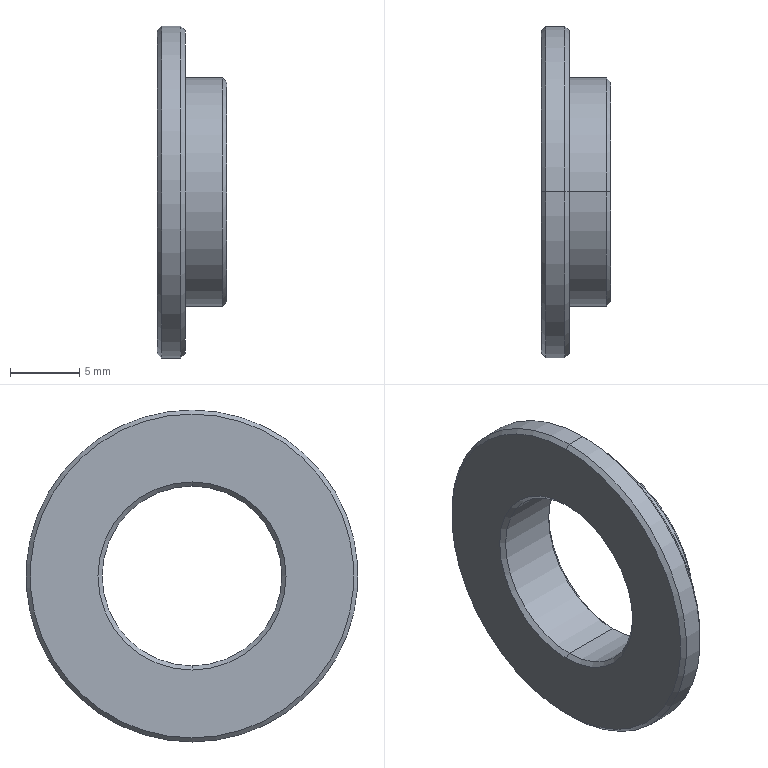Part | STEP file | ftcm_d16_5_h24_v13_0_t2_0_l5_0_2_03 | 1 solid | 19 faces | box 5 x 24 x 24 mm | volume 869.825 mm3 | cone 10 | cylinder 6 | plane 3 | commonest cylinder face diameters 13 x2 16.5 x2 24 x2
STEP:
#1=CARTESIAN_POINT('',(0.,0.,0.));
#2=DIRECTION('',(0.,0.,1.));
#3=DIRECTION('',(1.,0.,0.));
#4=AXIS2_PLACEMENT_3D('',#1,#2,#3);
#5=CARTESIAN_POINT('',(0.,0.,11.7));
#6=VERTEX_POINT('',#5);
#7=CARTESIAN_POINT('',(0.,0.,-11.7));
#8=VERTEX_POINT('',#7);
#9=CARTESIAN_POINT('',(0.,0.,0.));
#10=DIRECTION('',(-1.,0.,0.));
#11=DIRECTION('',(0.,0.,-1.));
#12=AXIS2_PLACEMENT_3D('',#9,#10,#11);
#13=CIRCLE('',#12,11.7);
#14=CARTESIAN_POINT('',(0.3,0.,0.));
#15=DIRECTION('',(1.,0.,0.));
#16=DIRECTION('',(0.,0.,-1.));
#17=AXIS2_PLACEMENT_3D('',#14,#15,#16);
#18=CONICAL_SURFACE('',#17,12.,0.7854);
#19=CARTESIAN_POINT('',(6.283,-0.3));
#20=DIRECTION('',(-1.,0.));
#21=VECTOR('',#20,1.);
#22=LINE('',#19,#21);
#23=(GEOMETRIC_REPRESENTATION_CONTEXT(2)PARAMETRIC_REPRESENTATION_CONTEXT()REPRESENTATION_CONTEXT('',''));
#24=DEFINITIONAL_REPRESENTATION('',(#22),#23);
#25=PCURVE('',#18,#24);
#26=CARTESIAN_POINT('',(0.,9.25,0.));
#27=DIRECTION('',(-1.,0.,0.));
#28=DIRECTION('',(0.,0.,1.));
#29=AXIS2_PLACEMENT_3D('',#26,#27,#28);
#30=PLANE('',#29);
#31=CARTESIAN_POINT('',(0.,-9.25));
#32=DIRECTION('',(-1.,0.));
#33=AXIS2_PLACEMENT_2D('',#31,#32);
#34=CIRCLE('',#33,11.7);
#35=(GEOMETRIC_REPRESENTATION_CONTEXT(2)PARAMETRIC_REPRESENTATION_CONTEXT()REPRESENTATION_CONTEXT('',''));
#36=DEFINITIONAL_REPRESENTATION('',(#34),#35);
#37=PCURVE('',#30,#36);
#38=SURFACE_CURVE('',#13,(#25,#37),.PCURVE_S1.);
#39=EDGE_CURVE('',#6,#8,#38,.T.);
#40=ORIENTED_EDGE('',*,*,#39,.F.);
#41=CARTESIAN_POINT('',(0.3,0.,12.));
#42=VERTEX_POINT('',#41);
#43=CARTESIAN_POINT('',(0.3,0.,12.));
#44=DIRECTION('',(0.7071,0.,0.7071));
#45=VECTOR('',#44,1.);
#46=LINE('',#43,#45);
#47=CARTESIAN_POINT('',(3.142,0.));
#48=DIRECTION('',(0.,1.));
#49=VECTOR('',#48,1.);
#50=LINE('',#47,#49);
#51=(GEOMETRIC_REPRESENTATION_CONTEXT(2)PARAMETRIC_REPRESENTATION_CONTEXT()REPRESENTATION_CONTEXT('',''));
#52=DEFINITIONAL_REPRESENTATION('',(#50),#51);
#53=PCURVE('',#18,#52);
#54=CARTESIAN_POINT('',(0.3,0.,0.));
#55=DIRECTION('',(1.,0.,0.));
#56=DIRECTION('',(0.,0.,-1.));
#57=AXIS2_PLACEMENT_3D('',#54,#55,#56);
#58=CONICAL_SURFACE('',#57,12.,0.7854);
#59=CARTESIAN_POINT('',(3.142,0.));
#60=DIRECTION('',(0.,1.));
#61=VECTOR('',#60,1.);
#62=LINE('',#59,#61);
#63=(GEOMETRIC_REPRESENTATION_CONTEXT(2)PARAMETRIC_REPRESENTATION_CONTEXT()REPRESENTATION_CONTEXT('',''));
#64=DEFINITIONAL_REPRESENTATION('',(#62),#63);
#65=PCURVE('',#58,#64);
#66=SURFACE_CURVE('',#46,(#53,#65),.PCURVE_S1.);
#67=EDGE_CURVE('',#6,#42,#66,.T.);
#68=ORIENTED_EDGE('',*,*,#67,.T.);
#69=CARTESIAN_POINT('',(0.3,0.,-12.));
#70=VERTEX_POINT('',#69);
#71=CARTESIAN_POINT('',(0.3,0.,0.));
#72=DIRECTION('',(-1.,0.,0.));
#73=DIRECTION('',(0.,1.,0.));
#74=AXIS2_PLACEMENT_3D('',#71,#72,#73);
#75=CIRCLE('',#74,12.);
#76=CARTESIAN_POINT('',(7.854,0.));
#77=DIRECTION('',(-1.,0.));
#78=VECTOR('',#77,1.);
#79=LINE('',#76,#78);
#80=(GEOMETRIC_REPRESENTATION_CONTEXT(2)PARAMETRIC_REPRESENTATION_CONTEXT()REPRESENTATION_CONTEXT('',''));
#81=DEFINITIONAL_REPRESENTATION('',(#79),#80);
#82=PCURVE('',#18,#81);
#83=CARTESIAN_POINT('',(1.,0.,0.));
#84=DIRECTION('',(1.,0.,0.));
#85=DIRECTION('',(0.,0.,-1.));
#86=AXIS2_PLACEMENT_3D('',#83,#84,#85);
#87=CYLINDRICAL_SURFACE('',#86,12.);
#88=CARTESIAN_POINT('',(7.854,-0.7));
#89=DIRECTION('',(-1.,0.));
#90=VECTOR('',#89,1.);
#91=LINE('',#88,#90);
#92=(GEOMETRIC_REPRESENTATION_CONTEXT(2)PARAMETRIC_REPRESENTATION_CONTEXT()REPRESENTATION_CONTEXT('',''));
#93=DEFINITIONAL_REPRESENTATION('',(#91),#92);
#94=PCURVE('',#87,#93);
#95=SURFACE_CURVE('',#75,(#82,#94),.PCURVE_S1.);
#96=EDGE_CURVE('',#42,#70,#95,.T.);
#97=ORIENTED_EDGE('',*,*,#96,.T.);
#98=CARTESIAN_POINT('',(0.3,0.,-12.));
#99=DIRECTION('',(0.7071,0.,-0.7071));
#100=VECTOR('',#99,1.);
#101=LINE('',#98,#100);
#102=CARTESIAN_POINT('',(0.,0.));
#103=DIRECTION('',(0.,1.));
#104=VECTOR('',#103,1.);
#105=LINE('',#102,#104);
#106=(GEOMETRIC_REPRESENTATION_CONTEXT(2)PARAMETRIC_REPRESENTATION_CONTEXT()REPRESENTATION_CONTEXT('',''));
#107=DEFINITIONAL_REPRESENTATION('',(#105),#106);
#108=PCURVE('',#18,#107);
#109=CARTESIAN_POINT('',(6.283,0.));
#110=DIRECTION('',(0.,1.));
#111=VECTOR('',#110,1.);
#112=LINE('',#109,#111);
#113=(GEOMETRIC_REPRESENTATION_CONTEXT(2)PARAMETRIC_REPRESENTATION_CONTEXT()REPRESENTATION_CONTEXT('',''));
#114=DEFINITIONAL_REPRESENTATION('',(#112),#113);
#115=PCURVE('',#58,#114);
#116=SURFACE_CURVE('',#101,(#108,#115),.PCURVE_S1.);
#117=EDGE_CURVE('',#8,#70,#116,.T.);
#118=ORIENTED_EDGE('',*,*,#117,.F.);
#119=EDGE_LOOP('',(#40,#68,#97,#118));
#120=FACE_BOUND('',#119,.T.);
#121=ADVANCED_FACE('',(#120),#18,.T.);
#122=CARTESIAN_POINT('',(0.3,0.,6.5));
#123=VERTEX_POINT('',#122);
#124=CARTESIAN_POINT('',(0.,0.,6.8));
#125=VERTEX_POINT('',#124);
#126=CARTESIAN_POINT('',(0.,0.,6.8));
#127=DIRECTION('',(-0.7071,0.,0.7071));
#128=VECTOR('',#127,1.);
#129=LINE('',#126,#128);
#130=CARTESIAN_POINT('',(0.,0.,0.));
#131=DIRECTION('',(-1.,0.,0.));
#132=DIRECTION('',(0.,0.,1.));
#133=AXIS2_PLACEMENT_3D('',#130,#131,#132);
#134=CONICAL_SURFACE('',#133,6.8,0.7854);
#135=CARTESIAN_POINT('',(6.283,0.));
#136=DIRECTION('',(0.,1.));
#137=VECTOR('',#136,1.);
#138=LINE('',#135,#137);
#139=(GEOMETRIC_REPRESENTATION_CONTEXT(2)PARAMETRIC_REPRESENTATION_CONTEXT()REPRESENTATION_CONTEXT('',''));
#140=DEFINITIONAL_REPRESENTATION('',(#138),#139);
#141=PCURVE('',#134,#140);
#142=CARTESIAN_POINT('',(0.,0.,0.));
#143=DIRECTION('',(-1.,0.,0.));
#144=DIRECTION('',(0.,0.,1.));
#145=AXIS2_PLACEMENT_3D('',#142,#143,#144);
#146=CONICAL_SURFACE('',#145,6.8,0.7854);
#147=CARTESIAN_POINT('',(0.,0.));
#148=DIRECTION('',(0.,1.));
#149=VECTOR('',#148,1.);
#150=LINE('',#147,#149);
#151=(GEOMETRIC_REPRESENTATION_CONTEXT(2)PARAMETRIC_REPRESENTATION_CONTEXT()REPRESENTATION_CONTEXT('',''));
#152=DEFINITIONAL_REPRESENTATION('',(#150),#151);
#153=PCURVE('',#146,#152);
#154=SURFACE_CURVE('',#129,(#141,#153),.PCURVE_S1.);
#155=EDGE_CURVE('',#123,#125,#154,.T.);
#156=ORIENTED_EDGE('',*,*,#155,.T.);
#157=CARTESIAN_POINT('',(0.,0.,-6.8));
#158=VERTEX_POINT('',#157);
#159=CARTESIAN_POINT('',(0.,0.,0.));
#160=DIRECTION('',(1.,0.,0.));
#161=DIRECTION('',(0.,0.,1.));
#162=AXIS2_PLACEMENT_3D('',#159,#160,#161);
#163=CIRCLE('',#162,6.8);
#164=CARTESIAN_POINT('',(6.283,0.));
#165=DIRECTION('',(-1.,0.));
#166=VECTOR('',#165,1.);
#167=LINE('',#164,#166);
#168=(GEOMETRIC_REPRESENTATION_CONTEXT(2)PARAMETRIC_REPRESENTATION_CONTEXT()REPRESENTATION_CONTEXT('',''));
#169=DEFINITIONAL_REPRESENTATION('',(#167),#168);
#170=PCURVE('',#134,#169);
#171=CARTESIAN_POINT('',(6.8,-9.25));
#172=CARTESIAN_POINT('',(6.8,-21.028));
#173=CARTESIAN_POINT('',(-3.4,-15.139));
#174=CARTESIAN_POINT('',(-13.6,-9.25));
#175=CARTESIAN_POINT('',(-3.4,-3.361));
#176=CARTESIAN_POINT('',(6.8,2.528));
#177=CARTESIAN_POINT('',(6.8,-9.25));
#178=(BOUNDED_CURVE()B_SPLINE_CURVE(2,(#171,#172,#173,#174,#175,#176,#177),.UNSPECIFIED.,.T.,.F.)B_SPLINE_CURVE_WITH_KNOTS((1,2,2,2,2,1),(-2.094,0.,2.094,4.189,6.283,8.378),.UNSPECIFIED.)CURVE()GEOMETRIC_REPRESENTATION_ITEM()RATIONAL_B_SPLINE_CURVE((1.,0.5,1.,0.5,1.,0.5,1.))REPRESENTATION_ITEM(''));
#179=(GEOMETRIC_REPRESENTATION_CONTEXT(2)PARAMETRIC_REPRESENTATION_CONTEXT()REPRESENTATION_CONTEXT('',''));
#180=DEFINITIONAL_REPRESENTATION('',(#178),#179);
#181=PCURVE('',#30,#180);
#182=SURFACE_CURVE('',#163,(#170,#181),.PCURVE_S1.);
#183=EDGE_CURVE('',#125,#158,#182,.T.);
#184=ORIENTED_EDGE('',*,*,#183,.T.);
#185=CARTESIAN_POINT('',(0.3,0.,-6.5));
#186=VERTEX_POINT('',#185);
#187=CARTESIAN_POINT('',(0.,0.,-6.8));
#188=DIRECTION('',(-0.7071,0.,-0.7071));
#189=VECTOR('',#188,1.);
#190=LINE('',#187,#189);
#191=CARTESIAN_POINT('',(3.142,0.));
#192=DIRECTION('',(0.,1.));
#193=VECTOR('',#192,1.);
#194=LINE('',#191,#193);
#195=(GEOMETRIC_REPRESENTATION_CONTEXT(2)PARAMETRIC_REPRESENTATION_CONTEXT()REPRESENTATION_CONTEXT('',''));
#196=DEFINITIONAL_REPRESENTATION('',(#194),#195);
#197=PCURVE('',#134,#196);
#198=CARTESIAN_POINT('',(3.142,0.));
#199=DIRECTION('',(0.,1.));
#200=VECTOR('',#199,1.);
#201=LINE('',#198,#200);
#202=(GEOMETRIC_REPRESENTATION_CONTEXT(2)PARAMETRIC_REPRESENTATION_CONTEXT()REPRESENTATION_CONTEXT('',''));
#203=DEFINITIONAL_REPRESENTATION('',(#201),#202);
#204=PCURVE('',#146,#203);
#205=SURFACE_CURVE('',#190,(#197,#204),.PCURVE_S1.);
#206=EDGE_CURVE('',#186,#158,#205,.T.);
#207=ORIENTED_EDGE('',*,*,#206,.F.);
#208=CARTESIAN_POINT('',(0.3,0.,0.));
#209=DIRECTION('',(-1.,0.,0.));
#210=DIRECTION('',(0.,1.,0.));
#211=AXIS2_PLACEMENT_3D('',#208,#209,#210);
#212=CIRCLE('',#211,6.5);
#213=CARTESIAN_POINT('',(1.571,-0.3));
#214=DIRECTION('',(1.,0.));
#215=VECTOR('',#214,1.);
#216=LINE('',#213,#215);
#217=(GEOMETRIC_REPRESENTATION_CONTEXT(2)PARAMETRIC_REPRESENTATION_CONTEXT()REPRESENTATION_CONTEXT('',''));
#218=DEFINITIONAL_REPRESENTATION('',(#216),#217);
#219=PCURVE('',#134,#218);
#220=CARTESIAN_POINT('',(2.5,0.,0.));
#221=DIRECTION('',(1.,0.,0.));
#222=DIRECTION('',(0.,0.,-1.));
#223=AXIS2_PLACEMENT_3D('',#220,#221,#222);
#224=CYLINDRICAL_SURFACE('',#223,6.5);
#225=CARTESIAN_POINT('',(7.854,-2.2));
#226=DIRECTION('',(-1.,0.));
#227=VECTOR('',#226,1.);
#228=LINE('',#225,#227);
#229=(GEOMETRIC_REPRESENTATION_CONTEXT(2)PARAMETRIC_REPRESENTATION_CONTEXT()REPRESENTATION_CONTEXT('',''));
#230=DEFINITIONAL_REPRESENTATION('',(#228),#229);
#231=PCURVE('',#224,#230);
#232=SURFACE_CURVE('',#212,(#219,#231),.PCURVE_S1.);
#233=EDGE_CURVE('',#186,#123,#232,.T.);
#234=ORIENTED_EDGE('',*,*,#233,.T.);
#235=EDGE_LOOP('',(#156,#184,#207,#234));
#236=FACE_BOUND('',#235,.F.);
#237=ADVANCED_FACE('',(#236),#134,.F.);
#238=ORIENTED_EDGE('',*,*,#96,.F.);
#239=CARTESIAN_POINT('',(1.7,0.,12.));
#240=VERTEX_POINT('',#239);
#241=CARTESIAN_POINT('',(1.,0.,12.));
#242=DIRECTION('',(1.,0.,0.));
#243=VECTOR('',#242,1.);
#244=LINE('',#241,#243);
#245=CARTESIAN_POINT('',(3.142,0.));
#246=DIRECTION('',(0.,1.));
#247=VECTOR('',#246,1.);
#248=LINE('',#245,#247);
#249=(GEOMETRIC_REPRESENTATION_CONTEXT(2)PARAMETRIC_REPRESENTATION_CONTEXT()REPRESENTATION_CONTEXT('',''));
#250=DEFINITIONAL_REPRESENTATION('',(#248),#249);
#251=PCURVE('',#87,#250);
#252=CARTESIAN_POINT('',(1.,0.,0.));
#253=DIRECTION('',(1.,0.,0.));
#254=DIRECTION('',(0.,0.,-1.));
#255=AXIS2_PLACEMENT_3D('',#252,#253,#254);
#256=CYLINDRICAL_SURFACE('',#255,12.);
#257=CARTESIAN_POINT('',(3.142,0.));
#258=DIRECTION('',(0.,1.));
#259=VECTOR('',#258,1.);
#260=LINE('',#257,#259);
#261=(GEOMETRIC_REPRESENTATION_CONTEXT(2)PARAMETRIC_REPRESENTATION_CONTEXT()REPRESENTATION_CONTEXT('',''));
#262=DEFINITIONAL_REPRESENTATION('',(#260),#261);
#263=PCURVE('',#256,#262);
#264=SURFACE_CURVE('',#244,(#251,#263),.PCURVE_S1.);
#265=EDGE_CURVE('',#42,#240,#264,.T.);
#266=ORIENTED_EDGE('',*,*,#265,.T.);
#267=CARTESIAN_POINT('',(1.7,0.,-12.));
#268=VERTEX_POINT('',#267);
#269=CARTESIAN_POINT('',(1.7,0.,0.));
#270=DIRECTION('',(-1.,0.,0.));
#271=DIRECTION('',(0.,0.,-1.));
#272=AXIS2_PLACEMENT_3D('',#269,#270,#271);
#273=CIRCLE('',#272,12.);
#274=CARTESIAN_POINT('',(6.283,0.7));
#275=DIRECTION('',(-1.,0.));
#276=VECTOR('',#275,1.);
#277=LINE('',#274,#276);
#278=(GEOMETRIC_REPRESENTATION_CONTEXT(2)PARAMETRIC_REPRESENTATION_CONTEXT()REPRESENTATION_CONTEXT('',''));
#279=DEFINITIONAL_REPRESENTATION('',(#277),#278);
#280=PCURVE('',#87,#279);
#281=CARTESIAN_POINT('',(1.7,0.,0.));
#282=DIRECTION('',(-1.,0.,0.));
#283=DIRECTION('',(0.,0.,1.));
#284=AXIS2_PLACEMENT_3D('',#281,#282,#283);
#285=CONICAL_SURFACE('',#284,12.,0.7854);
#286=CARTESIAN_POINT('',(-3.142,0.));
#287=DIRECTION('',(1.,0.));
#288=VECTOR('',#287,1.);
#289=LINE('',#286,#288);
#290=(GEOMETRIC_REPRESENTATION_CONTEXT(2)PARAMETRIC_REPRESENTATION_CONTEXT()REPRESENTATION_CONTEXT('',''));
#291=DEFINITIONAL_REPRESENTATION('',(#289),#290);
#292=PCURVE('',#285,#291);
#293=SURFACE_CURVE('',#273,(#280,#292),.PCURVE_S1.);
#294=EDGE_CURVE('',#240,#268,#293,.T.);
#295=ORIENTED_EDGE('',*,*,#294,.T.);
#296=CARTESIAN_POINT('',(1.,0.,-12.));
#297=DIRECTION('',(1.,0.,0.));
#298=VECTOR('',#297,1.);
#299=LINE('',#296,#298);
#300=CARTESIAN_POINT('',(0.,0.));
#301=DIRECTION('',(0.,1.));
#302=VECTOR('',#301,1.);
#303=LINE('',#300,#302);
#304=(GEOMETRIC_REPRESENTATION_CONTEXT(2)PARAMETRIC_REPRESENTATION_CONTEXT()REPRESENTATION_CONTEXT('',''));
#305=DEFINITIONAL_REPRESENTATION('',(#303),#304);
#306=PCURVE('',#87,#305);
#307=CARTESIAN_POINT('',(6.283,0.));
#308=DIRECTION('',(0.,1.));
#309=VECTOR('',#308,1.);
#310=LINE('',#307,#309);
#311=(GEOMETRIC_REPRESENTATION_CONTEXT(2)PARAMETRIC_REPRESENTATION_CONTEXT()REPRESENTATION_CONTEXT('',''));
#312=DEFINITIONAL_REPRESENTATION('',(#310),#311);
#313=PCURVE('',#256,#312);
#314=SURFACE_CURVE('',#299,(#306,#313),.PCURVE_S1.);
#315=EDGE_CURVE('',#70,#268,#314,.T.);
#316=ORIENTED_EDGE('',*,*,#315,.F.);
#317=EDGE_LOOP('',(#238,#266,#295,#316));
#318=FACE_BOUND('',#317,.T.);
#319=ADVANCED_FACE('',(#318),#87,.T.);
#320=CARTESIAN_POINT('',(4.7,0.,-6.5));
#321=VERTEX_POINT('',#320);
#322=CARTESIAN_POINT('',(2.5,0.,-6.5));
#323=DIRECTION('',(1.,0.,0.));
#324=VECTOR('',#323,1.);
#325=LINE('',#322,#324);
#326=CARTESIAN_POINT('',(6.283,0.));
#327=DIRECTION('',(0.,1.));
#328=VECTOR('',#327,1.);
#329=LINE('',#326,#328);
#330=(GEOMETRIC_REPRESENTATION_CONTEXT(2)PARAMETRIC_REPRESENTATION_CONTEXT()REPRESENTATION_CONTEXT('',''));
#331=DEFINITIONAL_REPRESENTATION('',(#329),#330);
#332=PCURVE('',#224,#331);
#333=CARTESIAN_POINT('',(2.5,0.,0.));
#334=DIRECTION('',(1.,0.,0.));
#335=DIRECTION('',(0.,0.,-1.));
#336=AXIS2_PLACEMENT_3D('',#333,#334,#335);
#337=CYLINDRICAL_SURFACE('',#336,6.5);
#338=CARTESIAN_POINT('',(0.,0.));
#339=DIRECTION('',(0.,1.));
#340=VECTOR('',#339,1.);
#341=LINE('',#338,#340);
#342=(GEOMETRIC_REPRESENTATION_CONTEXT(2)PARAMETRIC_REPRESENTATION_CONTEXT()REPRESENTATION_CONTEXT('',''));
#343=DEFINITIONAL_REPRESENTATION('',(#341),#342);
#344=PCURVE('',#337,#343);
#345=SURFACE_CURVE('',#325,(#332,#344),.PCURVE_S1.);
#346=EDGE_CURVE('',#186,#321,#345,.T.);
#347=ORIENTED_EDGE('',*,*,#346,.T.);
#348=CARTESIAN_POINT('',(4.7,0.,6.5));
#349=VERTEX_POINT('',#348);
#350=CARTESIAN_POINT('',(4.7,0.,0.));
#351=DIRECTION('',(-1.,0.,0.));
#352=DIRECTION('',(0.,0.,-1.));
#353=AXIS2_PLACEMENT_3D('',#350,#351,#352);
#354=CIRCLE('',#353,6.5);
#355=CARTESIAN_POINT('',(6.283,2.2));
#356=DIRECTION('',(-1.,0.));
#357=VECTOR('',#356,1.);
#358=LINE('',#355,#357);
#359=(GEOMETRIC_REPRESENTATION_CONTEXT(2)PARAMETRIC_REPRESENTATION_CONTEXT()REPRESENTATION_CONTEXT('',''));
#360=DEFINITIONAL_REPRESENTATION('',(#358),#359);
#361=PCURVE('',#224,#360);
#362=CARTESIAN_POINT('',(5.,0.,0.));
#363=DIRECTION('',(1.,0.,0.));
#364=DIRECTION('',(0.,0.,-1.));
#365=AXIS2_PLACEMENT_3D('',#362,#363,#364);
#366=CONICAL_SURFACE('',#365,6.8,0.7854);
#367=CARTESIAN_POINT('',(6.283,-0.3));
#368=DIRECTION('',(-1.,0.));
#369=VECTOR('',#368,1.);
#370=LINE('',#367,#369);
#371=(GEOMETRIC_REPRESENTATION_CONTEXT(2)PARAMETRIC_REPRESENTATION_CONTEXT()REPRESENTATION_CONTEXT('',''));
#372=DEFINITIONAL_REPRESENTATION('',(#370),#371);
#373=PCURVE('',#366,#372);
#374=SURFACE_CURVE('',#354,(#361,#373),.PCURVE_S1.);
#375=EDGE_CURVE('',#321,#349,#374,.T.);
#376=ORIENTED_EDGE('',*,*,#375,.T.);
#377=CARTESIAN_POINT('',(2.5,0.,6.5));
#378=DIRECTION('',(1.,0.,0.));
#379=VECTOR('',#378,1.);
#380=LINE('',#377,#379);
#381=CARTESIAN_POINT('',(3.142,0.));
#382=DIRECTION('',(0.,1.));
#383=VECTOR('',#382,1.);
#384=LINE('',#381,#383);
#385=(GEOMETRIC_REPRESENTATION_CONTEXT(2)PARAMETRIC_REPRESENTATION_CONTEXT()REPRESENTATION_CONTEXT('',''));
#386=DEFINITIONAL_REPRESENTATION('',(#384),#385);
#387=PCURVE('',#224,#386);
#388=CARTESIAN_POINT('',(3.142,0.));
#389=DIRECTION('',(0.,1.));
#390=VECTOR('',#389,1.);
#391=LINE('',#388,#390);
#392=(GEOMETRIC_REPRESENTATION_CONTEXT(2)PARAMETRIC_REPRESENTATION_CONTEXT()REPRESENTATION_CONTEXT('',''));
#393=DEFINITIONAL_REPRESENTATION('',(#391),#392);
#394=PCURVE('',#337,#393);
#395=SURFACE_CURVE('',#380,(#387,#394),.PCURVE_S1.);
#396=EDGE_CURVE('',#123,#349,#395,.T.);
#397=ORIENTED_EDGE('',*,*,#396,.F.);
#398=ORIENTED_EDGE('',*,*,#233,.F.);
#399=EDGE_LOOP('',(#347,#376,#397,#398));
#400=FACE_BOUND('',#399,.F.);
#401=ADVANCED_FACE('',(#400),#224,.F.);
#402=CARTESIAN_POINT('',(2.,0.,11.7));
#403=VERTEX_POINT('',#402);
#404=CARTESIAN_POINT('',(2.,0.,-11.7));
#405=VERTEX_POINT('',#404);
#406=CARTESIAN_POINT('',(2.,0.,0.));
#407=DIRECTION('',(-1.,0.,0.));
#408=DIRECTION('',(0.,0.,1.));
#409=AXIS2_PLACEMENT_3D('',#406,#407,#408);
#410=CIRCLE('',#409,11.7);
#411=CARTESIAN_POINT('',(0.,-0.3));
#412=DIRECTION('',(1.,0.));
#413=VECTOR('',#412,1.);
#414=LINE('',#411,#413);
#415=(GEOMETRIC_REPRESENTATION_CONTEXT(2)PARAMETRIC_REPRESENTATION_CONTEXT()REPRESENTATION_CONTEXT('',''));
#416=DEFINITIONAL_REPRESENTATION('',(#414),#415);
#417=PCURVE('',#285,#416);
#418=CARTESIAN_POINT('',(2.,9.975,0.));
#419=DIRECTION('',(1.,0.,0.));
#420=DIRECTION('',(0.,0.,-1.));
#421=AXIS2_PLACEMENT_3D('',#418,#419,#420);
#422=PLANE('',#421);
#423=CARTESIAN_POINT('',(-11.7,-9.975));
#424=CARTESIAN_POINT('',(-11.7,10.29));
#425=CARTESIAN_POINT('',(5.85,0.1575));
#426=CARTESIAN_POINT('',(23.4,-9.975));
#427=CARTESIAN_POINT('',(5.85,-20.107));
#428=CARTESIAN_POINT('',(-11.7,-30.24));
#429=CARTESIAN_POINT('',(-11.7,-9.975));
#430=(BOUNDED_CURVE()B_SPLINE_CURVE(2,(#423,#424,#425,#426,#427,#428,#429),.UNSPECIFIED.,.T.,.F.)B_SPLINE_CURVE_WITH_KNOTS((1,2,2,2,2,1),(-2.094,0.,2.094,4.189,6.283,8.378),.UNSPECIFIED.)CURVE()GEOMETRIC_REPRESENTATION_ITEM()RATIONAL_B_SPLINE_CURVE((1.,0.5,1.,0.5,1.,0.5,1.))REPRESENTATION_ITEM(''));
#431=(GEOMETRIC_REPRESENTATION_CONTEXT(2)PARAMETRIC_REPRESENTATION_CONTEXT()REPRESENTATION_CONTEXT('',''));
#432=DEFINITIONAL_REPRESENTATION('',(#430),#431);
#433=PCURVE('',#422,#432);
#434=SURFACE_CURVE('',#410,(#417,#433),.PCURVE_S1.);
#435=EDGE_CURVE('',#403,#405,#434,.T.);
#436=ORIENTED_EDGE('',*,*,#435,.T.);
#437=CARTESIAN_POINT('',(1.7,0.,-12.));
#438=DIRECTION('',(-0.7071,0.,-0.7071));
#439=VECTOR('',#438,1.);
#440=LINE('',#437,#439);
#441=CARTESIAN_POINT('',(3.142,0.));
#442=DIRECTION('',(0.,1.));
#443=VECTOR('',#442,1.);
#444=LINE('',#441,#443);
#445=(GEOMETRIC_REPRESENTATION_CONTEXT(2)PARAMETRIC_REPRESENTATION_CONTEXT()REPRESENTATION_CONTEXT('',''));
#446=DEFINITIONAL_REPRESENTATION('',(#444),#445);
#447=PCURVE('',#285,#446);
#448=CARTESIAN_POINT('',(1.7,0.,0.));
#449=DIRECTION('',(-1.,0.,0.));
#450=DIRECTION('',(0.,0.,1.));
#451=AXIS2_PLACEMENT_3D('',#448,#449,#450);
#452=CONICAL_SURFACE('',#451,12.,0.7854);
#453=CARTESIAN_POINT('',(3.142,0.));
#454=DIRECTION('',(0.,1.));
#455=VECTOR('',#454,1.);
#456=LINE('',#453,#455);
#457=(GEOMETRIC_REPRESENTATION_CONTEXT(2)PARAMETRIC_REPRESENTATION_CONTEXT()REPRESENTATION_CONTEXT('',''));
#458=DEFINITIONAL_REPRESENTATION('',(#456),#457);
#459=PCURVE('',#452,#458);
#460=SURFACE_CURVE('',#440,(#447,#459),.PCURVE_S1.);
#461=EDGE_CURVE('',#405,#268,#460,.T.);
#462=ORIENTED_EDGE('',*,*,#461,.T.);
#463=ORIENTED_EDGE('',*,*,#294,.F.);
#464=CARTESIAN_POINT('',(1.7,0.,12.));
#465=DIRECTION('',(-0.7071,0.,0.7071));
#466=VECTOR('',#465,1.);
#467=LINE('',#464,#466);
#468=CARTESIAN_POINT('',(0.,0.));
#469=DIRECTION('',(0.,1.));
#470=VECTOR('',#469,1.);
#471=LINE('',#468,#470);
#472=(GEOMETRIC_REPRESENTATION_CONTEXT(2)PARAMETRIC_REPRESENTATION_CONTEXT()REPRESENTATION_CONTEXT('',''));
#473=DEFINITIONAL_REPRESENTATION('',(#471),#472);
#474=PCURVE('',#285,#473);
#475=CARTESIAN_POINT('',(6.283,0.));
#476=DIRECTION('',(0.,1.));
#477=VECTOR('',#476,1.);
#478=LINE('',#475,#477);
#479=(GEOMETRIC_REPRESENTATION_CONTEXT(2)PARAMETRIC_REPRESENTATION_CONTEXT()REPRESENTATION_CONTEXT('',''));
#480=DEFINITIONAL_REPRESENTATION('',(#478),#479);
#481=PCURVE('',#452,#480);
#482=SURFACE_CURVE('',#467,(#474,#481),.PCURVE_S1.);
#483=EDGE_CURVE('',#403,#240,#482,.T.);
#484=ORIENTED_EDGE('',*,*,#483,.F.);
#485=EDGE_LOOP('',(#436,#462,#463,#484));
#486=FACE_BOUND('',#485,.T.);
#487=ADVANCED_FACE('',(#486),#285,.T.);
#488=CARTESIAN_POINT('',(5.,0.,-6.8));
#489=VERTEX_POINT('',#488);
#490=CARTESIAN_POINT('',(5.,0.,-6.8));
#491=DIRECTION('',(0.7071,0.,-0.7071));
#492=VECTOR('',#491,1.);
#493=LINE('',#490,#492);
#494=CARTESIAN_POINT('',(6.283,0.));
#495=DIRECTION('',(0.,1.));
#496=VECTOR('',#495,1.);
#497=LINE('',#494,#496);
#498=(GEOMETRIC_REPRESENTATION_CONTEXT(2)PARAMETRIC_REPRESENTATION_CONTEXT()REPRESENTATION_CONTEXT('',''));
#499=DEFINITIONAL_REPRESENTATION('',(#497),#498);
#500=PCURVE('',#366,#499);
#501=CARTESIAN_POINT('',(5.,0.,0.));
#502=DIRECTION('',(1.,0.,0.));
#503=DIRECTION('',(0.,0.,-1.));
#504=AXIS2_PLACEMENT_3D('',#501,#502,#503);
#505=CONICAL_SURFACE('',#504,6.8,0.7854);
#506=CARTESIAN_POINT('',(0.,0.));
#507=DIRECTION('',(0.,1.));
#508=VECTOR('',#507,1.);
#509=LINE('',#506,#508);
#510=(GEOMETRIC_REPRESENTATION_CONTEXT(2)PARAMETRIC_REPRESENTATION_CONTEXT()REPRESENTATION_CONTEXT('',''));
#511=DEFINITIONAL_REPRESENTATION('',(#509),#510);
#512=PCURVE('',#505,#511);
#513=SURFACE_CURVE('',#493,(#500,#512),.PCURVE_S1.);
#514=EDGE_CURVE('',#321,#489,#513,.T.);
#515=ORIENTED_EDGE('',*,*,#514,.T.);
#516=CARTESIAN_POINT('',(5.,0.,6.8));
#517=VERTEX_POINT('',#516);
#518=CARTESIAN_POINT('',(5.,0.,0.));
#519=DIRECTION('',(-1.,0.,0.));
#520=DIRECTION('',(0.,0.,-1.));
#521=AXIS2_PLACEMENT_3D('',#518,#519,#520);
#522=CIRCLE('',#521,6.8);
#523=CARTESIAN_POINT('',(6.283,0.));
#524=DIRECTION('',(-1.,0.));
#525=VECTOR('',#524,1.);
#526=LINE('',#523,#525);
#527=(GEOMETRIC_REPRESENTATION_CONTEXT(2)PARAMETRIC_REPRESENTATION_CONTEXT()REPRESENTATION_CONTEXT('',''));
#528=DEFINITIONAL_REPRESENTATION('',(#526),#527);
#529=PCURVE('',#366,#528);
#530=CARTESIAN_POINT('',(5.,7.375,0.));
#531=DIRECTION('',(1.,0.,0.));
#532=DIRECTION('',(0.,0.,-1.));
#533=AXIS2_PLACEMENT_3D('',#530,#531,#532);
#534=PLANE('',#533);
#535=CARTESIAN_POINT('',(6.8,-7.375));
#536=CARTESIAN_POINT('',(6.8,-19.153));
#537=CARTESIAN_POINT('',(-3.4,-13.264));
#538=CARTESIAN_POINT('',(-13.6,-7.375));
#539=CARTESIAN_POINT('',(-3.4,-1.486));
#540=CARTESIAN_POINT('',(6.8,4.403));
#541=CARTESIAN_POINT('',(6.8,-7.375));
#542=(BOUNDED_CURVE()B_SPLINE_CURVE(2,(#535,#536,#537,#538,#539,#540,#541),.UNSPECIFIED.,.T.,.F.)B_SPLINE_CURVE_WITH_KNOTS((1,2,2,2,2,1),(-2.094,0.,2.094,4.189,6.283,8.378),.UNSPECIFIED.)CURVE()GEOMETRIC_REPRESENTATION_ITEM()RATIONAL_B_SPLINE_CURVE((1.,0.5,1.,0.5,1.,0.5,1.))REPRESENTATION_ITEM(''));
#543=(GEOMETRIC_REPRESENTATION_CONTEXT(2)PARAMETRIC_REPRESENTATION_CONTEXT()REPRESENTATION_CONTEXT('',''));
#544=DEFINITIONAL_REPRESENTATION('',(#542),#543);
#545=PCURVE('',#534,#544);
#546=SURFACE_CURVE('',#522,(#529,#545),.PCURVE_S1.);
#547=EDGE_CURVE('',#489,#517,#546,.T.);
#548=ORIENTED_EDGE('',*,*,#547,.T.);
#549=CARTESIAN_POINT('',(5.,0.,6.8));
#550=DIRECTION('',(0.7071,0.,0.7071));
#551=VECTOR('',#550,1.);
#552=LINE('',#549,#551);
#553=CARTESIAN_POINT('',(3.142,0.));
#554=DIRECTION('',(0.,1.));
#555=VECTOR('',#554,1.);
#556=LINE('',#553,#555);
#557=(GEOMETRIC_REPRESENTATION_CONTEXT(2)PARAMETRIC_REPRESENTATION_CONTEXT()REPRESENTATION_CONTEXT('',''));
#558=DEFINITIONAL_REPRESENTATION('',(#556),#557);
#559=PCURVE('',#366,#558);
#560=CARTESIAN_POINT('',(3.142,0.));
#561=DIRECTION('',(0.,1.));
#562=VECTOR('',#561,1.);
#563=LINE('',#560,#562);
#564=(GEOMETRIC_REPRESENTATION_CONTEXT(2)PARAMETRIC_REPRESENTATION_CONTEXT()REPRESENTATION_CONTEXT('',''));
#565=DEFINITIONAL_REPRESENTATION('',(#563),#564);
#566=PCURVE('',#505,#565);
#567=SURFACE_CURVE('',#552,(#559,#566),.PCURVE_S1.);
#568=EDGE_CURVE('',#349,#517,#567,.T.);
#569=ORIENTED_EDGE('',*,*,#568,.F.);
#570=ORIENTED_EDGE('',*,*,#375,.F.);
#571=EDGE_LOOP('',(#515,#548,#569,#570));
#572=FACE_BOUND('',#571,.F.);
#573=ADVANCED_FACE('',(#572),#366,.F.);
#574=CARTESIAN_POINT('',(2.,0.,8.25));
#575=VERTEX_POINT('',#574);
#576=CARTESIAN_POINT('',(2.,0.,-8.25));
#577=VERTEX_POINT('',#576);
#578=CARTESIAN_POINT('',(2.,0.,0.));
#579=DIRECTION('',(-1.,0.,0.));
#580=DIRECTION('',(0.,0.,-1.));
#581=AXIS2_PLACEMENT_3D('',#578,#579,#580);
#582=CIRCLE('',#581,8.25);
#583=CARTESIAN_POINT('',(3.35,0.,0.));
#584=DIRECTION('',(1.,0.,0.));
#585=DIRECTION('',(0.,0.,-1.));
#586=AXIS2_PLACEMENT_3D('',#583,#584,#585);
#587=CYLINDRICAL_SURFACE('',#586,8.25);
#588=CARTESIAN_POINT('',(6.283,-1.35));
#589=DIRECTION('',(-1.,0.));
#590=VECTOR('',#589,1.);
#591=LINE('',#588,#590);
#592=(GEOMETRIC_REPRESENTATION_CONTEXT(2)PARAMETRIC_REPRESENTATION_CONTEXT()REPRESENTATION_CONTEXT('',''));
#593=DEFINITIONAL_REPRESENTATION('',(#591),#592);
#594=PCURVE('',#587,#593);
#595=CARTESIAN_POINT('',(8.25,-9.975));
#596=CARTESIAN_POINT('',(8.25,-24.264));
#597=CARTESIAN_POINT('',(-4.125,-17.12));
#598=CARTESIAN_POINT('',(-16.5,-9.975));
#599=CARTESIAN_POINT('',(-4.125,-2.83));
#600=CARTESIAN_POINT('',(8.25,4.314));
#601=CARTESIAN_POINT('',(8.25,-9.975));
#602=(BOUNDED_CURVE()B_SPLINE_CURVE(2,(#595,#596,#597,#598,#599,#600,#601),.UNSPECIFIED.,.T.,.F.)B_SPLINE_CURVE_WITH_KNOTS((1,2,2,2,2,1),(-2.094,0.,2.094,4.189,6.283,8.378),.UNSPECIFIED.)CURVE()GEOMETRIC_REPRESENTATION_ITEM()RATIONAL_B_SPLINE_CURVE((1.,0.5,1.,0.5,1.,0.5,1.))REPRESENTATION_ITEM(''));
#603=(GEOMETRIC_REPRESENTATION_CONTEXT(2)PARAMETRIC_REPRESENTATION_CONTEXT()REPRESENTATION_CONTEXT('',''));
#604=DEFINITIONAL_REPRESENTATION('',(#602),#603);
#605=PCURVE('',#422,#604);
#606=SURFACE_CURVE('',#582,(#594,#605),.PCURVE_S1.);
#607=EDGE_CURVE('',#575,#577,#606,.T.);
#608=ORIENTED_EDGE('',*,*,#607,.F.);
#609=CARTESIAN_POINT('',(4.7,0.,8.25));
#610=VERTEX_POINT('',#609);
#611=CARTESIAN_POINT('',(3.35,0.,8.25));
#612=DIRECTION('',(1.,0.,0.));
#613=VECTOR('',#612,1.);
#614=LINE('',#611,#613);
#615=CARTESIAN_POINT('',(3.142,0.));
#616=DIRECTION('',(0.,1.));
#617=VECTOR('',#616,1.);
#618=LINE('',#615,#617);
#619=(GEOMETRIC_REPRESENTATION_CONTEXT(2)PARAMETRIC_REPRESENTATION_CONTEXT()REPRESENTATION_CONTEXT('',''));
#620=DEFINITIONAL_REPRESENTATION('',(#618),#619);
#621=PCURVE('',#587,#620);
#622=CARTESIAN_POINT('',(3.35,0.,0.));
#623=DIRECTION('',(1.,0.,0.));
#624=DIRECTION('',(0.,0.,-1.));
#625=AXIS2_PLACEMENT_3D('',#622,#623,#624);
#626=CYLINDRICAL_SURFACE('',#625,8.25);
#627=CARTESIAN_POINT('',(3.142,0.));
#628=DIRECTION('',(0.,1.));
#629=VECTOR('',#628,1.);
#630=LINE('',#627,#629);
#631=(GEOMETRIC_REPRESENTATION_CONTEXT(2)PARAMETRIC_REPRESENTATION_CONTEXT()REPRESENTATION_CONTEXT('',''));
#632=DEFINITIONAL_REPRESENTATION('',(#630),#631);
#633=PCURVE('',#626,#632);
#634=SURFACE_CURVE('',#614,(#621,#633),.PCURVE_S1.);
#635=EDGE_CURVE('',#575,#610,#634,.T.);
#636=ORIENTED_EDGE('',*,*,#635,.T.);
#637=CARTESIAN_POINT('',(4.7,0.,-8.25));
#638=VERTEX_POINT('',#637);
#639=CARTESIAN_POINT('',(4.7,0.,0.));
#640=DIRECTION('',(-1.,0.,0.));
#641=DIRECTION('',(0.,0.,-1.));
#642=AXIS2_PLACEMENT_3D('',#639,#640,#641);
#643=CIRCLE('',#642,8.25);
#644=CARTESIAN_POINT('',(6.283,1.35));
#645=DIRECTION('',(-1.,0.));
#646=VECTOR('',#645,1.);
#647=LINE('',#644,#646);
#648=(GEOMETRIC_REPRESENTATION_CONTEXT(2)PARAMETRIC_REPRESENTATION_CONTEXT()REPRESENTATION_CONTEXT('',''));
#649=DEFINITIONAL_REPRESENTATION('',(#647),#648);
#650=PCURVE('',#587,#649);
#651=CARTESIAN_POINT('',(4.7,0.,0.));
#652=DIRECTION('',(-1.,0.,0.));
#653=DIRECTION('',(0.,0.,1.));
#654=AXIS2_PLACEMENT_3D('',#651,#652,#653);
#655=CONICAL_SURFACE('',#654,8.25,0.7854);
#656=CARTESIAN_POINT('',(-3.142,0.));
#657=DIRECTION('',(1.,0.));
#658=VECTOR('',#657,1.);
#659=LINE('',#656,#658);
#660=(GEOMETRIC_REPRESENTATION_CONTEXT(2)PARAMETRIC_REPRESENTATION_CONTEXT()REPRESENTATION_CONTEXT('',''));
#661=DEFINITIONAL_REPRESENTATION('',(#659),#660);
#662=PCURVE('',#655,#661);
#663=SURFACE_CURVE('',#643,(#650,#662),.PCURVE_S1.);
#664=EDGE_CURVE('',#610,#638,#663,.T.);
#665=ORIENTED_EDGE('',*,*,#664,.T.);
#666=CARTESIAN_POINT('',(3.35,0.,-8.25));
#667=DIRECTION('',(1.,0.,0.));
#668=VECTOR('',#667,1.);
#669=LINE('',#666,#668);
#670=CARTESIAN_POINT('',(0.,0.));
#671=DIRECTION('',(0.,1.));
#672=VECTOR('',#671,1.);
#673=LINE('',#670,#672);
#674=(GEOMETRIC_REPRESENTATION_CONTEXT(2)PARAMETRIC_REPRESENTATION_CONTEXT()REPRESENTATION_CONTEXT('',''));
#675=DEFINITIONAL_REPRESENTATION('',(#673),#674);
#676=PCURVE('',#587,#675);
#677=CARTESIAN_POINT('',(6.283,0.));
#678=DIRECTION('',(0.,1.));
#679=VECTOR('',#678,1.);
#680=LINE('',#677,#679);
#681=(GEOMETRIC_REPRESENTATION_CONTEXT(2)PARAMETRIC_REPRESENTATION_CONTEXT()REPRESENTATION_CONTEXT('',''));
#682=DEFINITIONAL_REPRESENTATION('',(#680),#681);
#683=PCURVE('',#626,#682);
#684=SURFACE_CURVE('',#669,(#676,#683),.PCURVE_S1.);
#685=EDGE_CURVE('',#577,#638,#684,.T.);
#686=ORIENTED_EDGE('',*,*,#685,.F.);
#687=EDGE_LOOP('',(#608,#636,#665,#686));
#688=FACE_BOUND('',#687,.T.);
#689=ADVANCED_FACE('',(#688),#587,.T.);
#690=CARTESIAN_POINT('',(5.,0.,-7.95));
#691=VERTEX_POINT('',#690);
#692=CARTESIAN_POINT('',(5.,0.,7.95));
#693=VERTEX_POINT('',#692);
#694=CARTESIAN_POINT('',(5.,0.,0.));
#695=DIRECTION('',(1.,0.,0.));
#696=DIRECTION('',(0.,0.,1.));
#697=AXIS2_PLACEMENT_3D('',#694,#695,#696);
#698=CIRCLE('',#697,7.95);
#699=CARTESIAN_POINT('',(6.283,-0.3));
#700=DIRECTION('',(-1.,0.));
#701=VECTOR('',#700,1.);
#702=LINE('',#699,#701);
#703=(GEOMETRIC_REPRESENTATION_CONTEXT(2)PARAMETRIC_REPRESENTATION_CONTEXT()REPRESENTATION_CONTEXT('',''));
#704=DEFINITIONAL_REPRESENTATION('',(#702),#703);
#705=PCURVE('',#655,#704);
#706=CARTESIAN_POINT('',(0.,-7.375));
#707=DIRECTION('',(-1.,0.));
#708=AXIS2_PLACEMENT_2D('',#706,#707);
#709=CIRCLE('',#708,7.95);
#710=(GEOMETRIC_REPRESENTATION_CONTEXT(2)PARAMETRIC_REPRESENTATION_CONTEXT()REPRESENTATION_CONTEXT('',''));
#711=DEFINITIONAL_REPRESENTATION('',(#709),#710);
#712=PCURVE('',#534,#711);
#713=SURFACE_CURVE('',#698,(#705,#712),.PCURVE_S1.);
#714=EDGE_CURVE('',#691,#693,#713,.T.);
#715=ORIENTED_EDGE('',*,*,#714,.F.);
#716=CARTESIAN_POINT('',(4.7,0.,-8.25));
#717=DIRECTION('',(-0.7071,0.,-0.7071));
#718=VECTOR('',#717,1.);
#719=LINE('',#716,#718);
#720=CARTESIAN_POINT('',(3.142,0.));
#721=DIRECTION('',(0.,1.));
#722=VECTOR('',#721,1.);
#723=LINE('',#720,#722);
#724=(GEOMETRIC_REPRESENTATION_CONTEXT(2)PARAMETRIC_REPRESENTATION_CONTEXT()REPRESENTATION_CONTEXT('',''));
#725=DEFINITIONAL_REPRESENTATION('',(#723),#724);
#726=PCURVE('',#655,#725);
#727=CARTESIAN_POINT('',(4.7,0.,0.));
#728=DIRECTION('',(-1.,0.,0.));
#729=DIRECTION('',(0.,0.,1.));
#730=AXIS2_PLACEMENT_3D('',#727,#728,#729);
#731=CONICAL_SURFACE('',#730,8.25,0.7854);
#732=CARTESIAN_POINT('',(3.142,0.));
#733=DIRECTION('',(0.,1.));
#734=VECTOR('',#733,1.);
#735=LINE('',#732,#734);
#736=(GEOMETRIC_REPRESENTATION_CONTEXT(2)PARAMETRIC_REPRESENTATION_CONTEXT()REPRESENTATION_CONTEXT('',''));
#737=DEFINITIONAL_REPRESENTATION('',(#735),#736);
#738=PCURVE('',#731,#737);
#739=SURFACE_CURVE('',#719,(#726,#738),.PCURVE_S1.);
#740=EDGE_CURVE('',#691,#638,#739,.T.);
#741=ORIENTED_EDGE('',*,*,#740,.T.);
#742=ORIENTED_EDGE('',*,*,#664,.F.);
#743=CARTESIAN_POINT('',(4.7,0.,8.25));
#744=DIRECTION('',(-0.7071,0.,0.7071));
#745=VECTOR('',#744,1.);
#746=LINE('',#743,#745);
#747=CARTESIAN_POINT('',(0.,0.));
#748=DIRECTION('',(0.,1.));
#749=VECTOR('',#748,1.);
#750=LINE('',#747,#749);
#751=(GEOMETRIC_REPRESENTATION_CONTEXT(2)PARAMETRIC_REPRESENTATION_CONTEXT()REPRESENTATION_CONTEXT('',''));
#752=DEFINITIONAL_REPRESENTATION('',(#750),#751);
#753=PCURVE('',#655,#752);
#754=CARTESIAN_POINT('',(6.283,0.));
#755=DIRECTION('',(0.,1.));
#756=VECTOR('',#755,1.);
#757=LINE('',#754,#756);
#758=(GEOMETRIC_REPRESENTATION_CONTEXT(2)PARAMETRIC_REPRESENTATION_CONTEXT()REPRESENTATION_CONTEXT('',''));
#759=DEFINITIONAL_REPRESENTATION('',(#757),#758);
#760=PCURVE('',#731,#759);
#761=SURFACE_CURVE('',#746,(#753,#760),.PCURVE_S1.);
#762=EDGE_CURVE('',#693,#610,#761,.T.);
#763=ORIENTED_EDGE('',*,*,#762,.F.);
#764=EDGE_LOOP('',(#715,#741,#742,#763));
#765=FACE_BOUND('',#764,.T.);
#766=ADVANCED_FACE('',(#765),#655,.T.);
#767=CARTESIAN_POINT('',(0.,0.,0.));
#768=DIRECTION('',(-1.,0.,0.));
#769=DIRECTION('',(0.,0.,-1.));
#770=AXIS2_PLACEMENT_3D('',#767,#768,#769);
#771=CIRCLE('',#770,11.7);
#772=CARTESIAN_POINT('',(0.,-9.25));
#773=DIRECTION('',(-1.,0.));
#774=AXIS2_PLACEMENT_2D('',#772,#773);
#775=CIRCLE('',#774,11.7);
#776=(GEOMETRIC_REPRESENTATION_CONTEXT(2)PARAMETRIC_REPRESENTATION_CONTEXT()REPRESENTATION_CONTEXT('',''));
#777=DEFINITIONAL_REPRESENTATION('',(#775),#776);
#778=PCURVE('',#30,#777);
#779=CARTESIAN_POINT('',(6.283,-0.3));
#780=DIRECTION('',(-1.,0.));
#781=VECTOR('',#780,1.);
#782=LINE('',#779,#781);
#783=(GEOMETRIC_REPRESENTATION_CONTEXT(2)PARAMETRIC_REPRESENTATION_CONTEXT()REPRESENTATION_CONTEXT('',''));
#784=DEFINITIONAL_REPRESENTATION('',(#782),#783);
#785=PCURVE('',#58,#784);
#786=SURFACE_CURVE('',#771,(#778,#785),.PCURVE_S1.);
#787=EDGE_CURVE('',#8,#6,#786,.T.);
#788=ORIENTED_EDGE('',*,*,#787,.T.);
#789=ORIENTED_EDGE('',*,*,#39,.T.);
#790=EDGE_LOOP('',(#788,#789));
#791=FACE_BOUND('',#790,.T.);
#792=ORIENTED_EDGE('',*,*,#183,.T.);
#793=CARTESIAN_POINT('',(0.,0.,0.));
#794=DIRECTION('',(1.,0.,0.));
#795=DIRECTION('',(0.,0.,1.));
#796=AXIS2_PLACEMENT_3D('',#793,#794,#795);
#797=CIRCLE('',#796,6.8);
#798=CARTESIAN_POINT('',(6.8,-9.25));
#799=CARTESIAN_POINT('',(6.8,-21.028));
#800=CARTESIAN_POINT('',(-3.4,-15.139));
#801=CARTESIAN_POINT('',(-13.6,-9.25));
#802=CARTESIAN_POINT('',(-3.4,-3.361));
#803=CARTESIAN_POINT('',(6.8,2.528));
#804=CARTESIAN_POINT('',(6.8,-9.25));
#805=(BOUNDED_CURVE()B_SPLINE_CURVE(2,(#798,#799,#800,#801,#802,#803,#804),.UNSPECIFIED.,.T.,.F.)B_SPLINE_CURVE_WITH_KNOTS((1,2,2,2,2,1),(-2.094,0.,2.094,4.189,6.283,8.378),.UNSPECIFIED.)CURVE()GEOMETRIC_REPRESENTATION_ITEM()RATIONAL_B_SPLINE_CURVE((1.,0.5,1.,0.5,1.,0.5,1.))REPRESENTATION_ITEM(''));
#806=(GEOMETRIC_REPRESENTATION_CONTEXT(2)PARAMETRIC_REPRESENTATION_CONTEXT()REPRESENTATION_CONTEXT('',''));
#807=DEFINITIONAL_REPRESENTATION('',(#805),#806);
#808=PCURVE('',#30,#807);
#809=CARTESIAN_POINT('',(6.283,0.));
#810=DIRECTION('',(-1.,0.));
#811=VECTOR('',#810,1.);
#812=LINE('',#809,#811);
#813=(GEOMETRIC_REPRESENTATION_CONTEXT(2)PARAMETRIC_REPRESENTATION_CONTEXT()REPRESENTATION_CONTEXT('',''));
#814=DEFINITIONAL_REPRESENTATION('',(#812),#813);
#815=PCURVE('',#146,#814);
#816=SURFACE_CURVE('',#797,(#808,#815),.PCURVE_S1.);
#817=EDGE_CURVE('',#158,#125,#816,.T.);
#818=ORIENTED_EDGE('',*,*,#817,.T.);
#819=EDGE_LOOP('',(#792,#818));
#820=FACE_BOUND('',#819,.T.);
#821=ADVANCED_FACE('',(#791,#820),#30,.T.);
#822=ORIENTED_EDGE('',*,*,#67,.F.);
#823=ORIENTED_EDGE('',*,*,#787,.F.);
#824=ORIENTED_EDGE('',*,*,#117,.T.);
#825=CARTESIAN_POINT('',(0.3,0.,0.));
#826=DIRECTION('',(-1.,0.,0.));
#827=DIRECTION('',(0.,1.,0.));
#828=AXIS2_PLACEMENT_3D('',#825,#826,#827);
#829=CIRCLE('',#828,12.);
#830=CARTESIAN_POINT('',(7.854,0.));
#831=DIRECTION('',(-1.,0.));
#832=VECTOR('',#831,1.);
#833=LINE('',#830,#832);
#834=(GEOMETRIC_REPRESENTATION_CONTEXT(2)PARAMETRIC_REPRESENTATION_CONTEXT()REPRESENTATION_CONTEXT('',''));
#835=DEFINITIONAL_REPRESENTATION('',(#833),#834);
#836=PCURVE('',#58,#835);
#837=CARTESIAN_POINT('',(7.854,-0.7));
#838=DIRECTION('',(-1.,0.));
#839=VECTOR('',#838,1.);
#840=LINE('',#837,#839);
#841=(GEOMETRIC_REPRESENTATION_CONTEXT(2)PARAMETRIC_REPRESENTATION_CONTEXT()REPRESENTATION_CONTEXT('',''));
#842=DEFINITIONAL_REPRESENTATION('',(#840),#841);
#843=PCURVE('',#256,#842);
#844=SURFACE_CURVE('',#829,(#836,#843),.PCURVE_S1.);
#845=EDGE_CURVE('',#70,#42,#844,.T.);
#846=ORIENTED_EDGE('',*,*,#845,.T.);
#847=EDGE_LOOP('',(#822,#823,#824,#846));
#848=FACE_BOUND('',#847,.T.);
#849=ADVANCED_FACE('',(#848),#58,.T.);
#850=ORIENTED_EDGE('',*,*,#817,.T.);
#851=ORIENTED_EDGE('',*,*,#155,.F.);
#852=CARTESIAN_POINT('',(0.3,0.,0.));
#853=DIRECTION('',(-1.,0.,0.));
#854=DIRECTION('',(0.,1.,0.));
#855=AXIS2_PLACEMENT_3D('',#852,#853,#854);
#856=CIRCLE('',#855,6.5);
#857=CARTESIAN_POINT('',(-4.712,-0.3));
#858=DIRECTION('',(1.,0.));
#859=VECTOR('',#858,1.);
#860=LINE('',#857,#859);
#861=(GEOMETRIC_REPRESENTATION_CONTEXT(2)PARAMETRIC_REPRESENTATION_CONTEXT()REPRESENTATION_CONTEXT('',''));
#862=DEFINITIONAL_REPRESENTATION('',(#860),#861);
#863=PCURVE('',#146,#862);
#864=CARTESIAN_POINT('',(7.854,-2.2));
#865=DIRECTION('',(-1.,0.));
#866=VECTOR('',#865,1.);
#867=LINE('',#864,#866);
#868=(GEOMETRIC_REPRESENTATION_CONTEXT(2)PARAMETRIC_REPRESENTATION_CONTEXT()REPRESENTATION_CONTEXT('',''));
#869=DEFINITIONAL_REPRESENTATION('',(#867),#868);
#870=PCURVE('',#337,#869);
#871=SURFACE_CURVE('',#856,(#863,#870),.PCURVE_S1.);
#872=EDGE_CURVE('',#123,#186,#871,.T.);
#873=ORIENTED_EDGE('',*,*,#872,.T.);
#874=ORIENTED_EDGE('',*,*,#206,.T.);
#875=EDGE_LOOP('',(#850,#851,#873,#874));
#876=FACE_BOUND('',#875,.F.);
#877=ADVANCED_FACE('',(#876),#146,.F.);
#878=ORIENTED_EDGE('',*,*,#265,.F.);
#879=ORIENTED_EDGE('',*,*,#845,.F.);
#880=ORIENTED_EDGE('',*,*,#315,.T.);
#881=CARTESIAN_POINT('',(1.7,0.,0.));
#882=DIRECTION('',(-1.,0.,0.));
#883=DIRECTION('',(0.,0.,-1.));
#884=AXIS2_PLACEMENT_3D('',#881,#882,#883);
#885=CIRCLE('',#884,12.);
#886=CARTESIAN_POINT('',(6.283,0.7));
#887=DIRECTION('',(-1.,0.));
#888=VECTOR('',#887,1.);
#889=LINE('',#886,#888);
#890=(GEOMETRIC_REPRESENTATION_CONTEXT(2)PARAMETRIC_REPRESENTATION_CONTEXT()REPRESENTATION_CONTEXT('',''));
#891=DEFINITIONAL_REPRESENTATION('',(#889),#890);
#892=PCURVE('',#256,#891);
#893=CARTESIAN_POINT('',(3.142,0.));
#894=DIRECTION('',(1.,0.));
#895=VECTOR('',#894,1.);
#896=LINE('',#893,#895);
#897=(GEOMETRIC_REPRESENTATION_CONTEXT(2)PARAMETRIC_REPRESENTATION_CONTEXT()REPRESENTATION_CONTEXT('',''));
#898=DEFINITIONAL_REPRESENTATION('',(#896),#897);
#899=PCURVE('',#452,#898);
#900=SURFACE_CURVE('',#885,(#892,#899),.PCURVE_S1.);
#901=EDGE_CURVE('',#268,#240,#900,.T.);
#902=ORIENTED_EDGE('',*,*,#901,.T.);
#903=EDGE_LOOP('',(#878,#879,#880,#902));
#904=FACE_BOUND('',#903,.T.);
#905=ADVANCED_FACE('',(#904),#256,.T.);
#906=CARTESIAN_POINT('',(4.7,0.,0.));
#907=DIRECTION('',(-1.,0.,0.));
#908=DIRECTION('',(0.,0.,-1.));
#909=AXIS2_PLACEMENT_3D('',#906,#907,#908);
#910=CIRCLE('',#909,6.5);
#911=CARTESIAN_POINT('',(6.283,2.2));
#912=DIRECTION('',(-1.,0.));
#913=VECTOR('',#912,1.);
#914=LINE('',#911,#913);
#915=(GEOMETRIC_REPRESENTATION_CONTEXT(2)PARAMETRIC_REPRESENTATION_CONTEXT()REPRESENTATION_CONTEXT('',''));
#916=DEFINITIONAL_REPRESENTATION('',(#914),#915);
#917=PCURVE('',#337,#916);
#918=CARTESIAN_POINT('',(6.283,-0.3));
#919=DIRECTION('',(-1.,0.));
#920=VECTOR('',#919,1.);
#921=LINE('',#918,#920);
#922=(GEOMETRIC_REPRESENTATION_CONTEXT(2)PARAMETRIC_REPRESENTATION_CONTEXT()REPRESENTATION_CONTEXT('',''));
#923=DEFINITIONAL_REPRESENTATION('',(#921),#922);
#924=PCURVE('',#505,#923);
#925=SURFACE_CURVE('',#910,(#917,#924),.PCURVE_S1.);
#926=EDGE_CURVE('',#349,#321,#925,.T.);
#927=ORIENTED_EDGE('',*,*,#926,.T.);
#928=ORIENTED_EDGE('',*,*,#346,.F.);
#929=ORIENTED_EDGE('',*,*,#872,.F.);
#930=ORIENTED_EDGE('',*,*,#396,.T.);
#931=EDGE_LOOP('',(#927,#928,#929,#930));
#932=FACE_BOUND('',#931,.F.);
#933=ADVANCED_FACE('',(#932),#337,.F.);
#934=ORIENTED_EDGE('',*,*,#461,.F.);
#935=CARTESIAN_POINT('',(2.,0.,0.));
#936=DIRECTION('',(-1.,0.,0.));
#937=DIRECTION('',(0.,0.,1.));
#938=AXIS2_PLACEMENT_3D('',#935,#936,#937);
#939=CIRCLE('',#938,11.7);
#940=CARTESIAN_POINT('',(0.,-0.3));
#941=DIRECTION('',(1.,0.));
#942=VECTOR('',#941,1.);
#943=LINE('',#940,#942);
#944=(GEOMETRIC_REPRESENTATION_CONTEXT(2)PARAMETRIC_REPRESENTATION_CONTEXT()REPRESENTATION_CONTEXT('',''));
#945=DEFINITIONAL_REPRESENTATION('',(#943),#944);
#946=PCURVE('',#452,#945);
#947=CARTESIAN_POINT('',(-11.7,-9.975));
#948=CARTESIAN_POINT('',(-11.7,10.29));
#949=CARTESIAN_POINT('',(5.85,0.1575));
#950=CARTESIAN_POINT('',(23.4,-9.975));
#951=CARTESIAN_POINT('',(5.85,-20.107));
#952=CARTESIAN_POINT('',(-11.7,-30.24));
#953=CARTESIAN_POINT('',(-11.7,-9.975));
#954=(BOUNDED_CURVE()B_SPLINE_CURVE(2,(#947,#948,#949,#950,#951,#952,#953),.UNSPECIFIED.,.T.,.F.)B_SPLINE_CURVE_WITH_KNOTS((1,2,2,2,2,1),(-2.094,0.,2.094,4.189,6.283,8.378),.UNSPECIFIED.)CURVE()GEOMETRIC_REPRESENTATION_ITEM()RATIONAL_B_SPLINE_CURVE((1.,0.5,1.,0.5,1.,0.5,1.))REPRESENTATION_ITEM(''));
#955=(GEOMETRIC_REPRESENTATION_CONTEXT(2)PARAMETRIC_REPRESENTATION_CONTEXT()REPRESENTATION_CONTEXT('',''));
#956=DEFINITIONAL_REPRESENTATION('',(#954),#955);
#957=PCURVE('',#422,#956);
#958=SURFACE_CURVE('',#939,(#946,#957),.PCURVE_S1.);
#959=EDGE_CURVE('',#405,#403,#958,.T.);
#960=ORIENTED_EDGE('',*,*,#959,.T.);
#961=ORIENTED_EDGE('',*,*,#483,.T.);
#962=ORIENTED_EDGE('',*,*,#901,.F.);
#963=EDGE_LOOP('',(#934,#960,#961,#962));
#964=FACE_BOUND('',#963,.T.);
#965=ADVANCED_FACE('',(#964),#452,.T.);
#966=CARTESIAN_POINT('',(5.,0.,0.));
#967=DIRECTION('',(-1.,0.,0.));
#968=DIRECTION('',(0.,0.,-1.));
#969=AXIS2_PLACEMENT_3D('',#966,#967,#968);
#970=CIRCLE('',#969,6.8);
#971=CARTESIAN_POINT('',(6.283,0.));
#972=DIRECTION('',(-1.,0.));
#973=VECTOR('',#972,1.);
#974=LINE('',#971,#973);
#975=(GEOMETRIC_REPRESENTATION_CONTEXT(2)PARAMETRIC_REPRESENTATION_CONTEXT()REPRESENTATION_CONTEXT('',''));
#976=DEFINITIONAL_REPRESENTATION('',(#974),#975);
#977=PCURVE('',#505,#976);
#978=CARTESIAN_POINT('',(6.8,-7.375));
#979=CARTESIAN_POINT('',(6.8,-19.153));
#980=CARTESIAN_POINT('',(-3.4,-13.264));
#981=CARTESIAN_POINT('',(-13.6,-7.375));
#982=CARTESIAN_POINT('',(-3.4,-1.486));
#983=CARTESIAN_POINT('',(6.8,4.403));
#984=CARTESIAN_POINT('',(6.8,-7.375));
#985=(BOUNDED_CURVE()B_SPLINE_CURVE(2,(#978,#979,#980,#981,#982,#983,#984),.UNSPECIFIED.,.T.,.F.)B_SPLINE_CURVE_WITH_KNOTS((1,2,2,2,2,1),(-2.094,0.,2.094,4.189,6.283,8.378),.UNSPECIFIED.)CURVE()GEOMETRIC_REPRESENTATION_ITEM()RATIONAL_B_SPLINE_CURVE((1.,0.5,1.,0.5,1.,0.5,1.))REPRESENTATION_ITEM(''));
#986=(GEOMETRIC_REPRESENTATION_CONTEXT(2)PARAMETRIC_REPRESENTATION_CONTEXT()REPRESENTATION_CONTEXT('',''));
#987=DEFINITIONAL_REPRESENTATION('',(#985),#986);
#988=PCURVE('',#534,#987);
#989=SURFACE_CURVE('',#970,(#977,#988),.PCURVE_S1.);
#990=EDGE_CURVE('',#517,#489,#989,.T.);
#991=ORIENTED_EDGE('',*,*,#990,.T.);
#992=ORIENTED_EDGE('',*,*,#514,.F.);
#993=ORIENTED_EDGE('',*,*,#926,.F.);
#994=ORIENTED_EDGE('',*,*,#568,.T.);
#995=EDGE_LOOP('',(#991,#992,#993,#994));
#996=FACE_BOUND('',#995,.F.);
#997=ADVANCED_FACE('',(#996),#505,.F.);
#998=CARTESIAN_POINT('',(2.,0.,0.));
#999=DIRECTION('',(-1.,0.,0.));
#1000=DIRECTION('',(0.,0.,-1.));
#1001=AXIS2_PLACEMENT_3D('',#998,#999,#1000);
#1002=CIRCLE('',#1001,8.25);
#1003=CARTESIAN_POINT('',(8.25,-9.975));
#1004=CARTESIAN_POINT('',(8.25,-24.264));
#1005=CARTESIAN_POINT('',(-4.125,-17.12));
#1006=CARTESIAN_POINT('',(-16.5,-9.975));
#1007=CARTESIAN_POINT('',(-4.125,-2.83));
#1008=CARTESIAN_POINT('',(8.25,4.314));
#1009=CARTESIAN_POINT('',(8.25,-9.975));
#1010=(BOUNDED_CURVE()B_SPLINE_CURVE(2,(#1003,#1004,#1005,#1006,#1007,#1008,#1009),.UNSPECIFIED.,.T.,.F.)B_SPLINE_CURVE_WITH_KNOTS((1,2,2,2,2,1),(-2.094,0.,2.094,4.189,6.283,8.378),.UNSPECIFIED.)CURVE()GEOMETRIC_REPRESENTATION_ITEM()RATIONAL_B_SPLINE_CURVE((1.,0.5,1.,0.5,1.,0.5,1.))REPRESENTATION_ITEM(''));
#1011=(GEOMETRIC_REPRESENTATION_CONTEXT(2)PARAMETRIC_REPRESENTATION_CONTEXT()REPRESENTATION_CONTEXT('',''));
#1012=DEFINITIONAL_REPRESENTATION('',(#1010),#1011);
#1013=PCURVE('',#422,#1012);
#1014=CARTESIAN_POINT('',(6.283,-1.35));
#1015=DIRECTION('',(-1.,0.));
#1016=VECTOR('',#1015,1.);
#1017=LINE('',#1014,#1016);
#1018=(GEOMETRIC_REPRESENTATION_CONTEXT(2)PARAMETRIC_REPRESENTATION_CONTEXT()REPRESENTATION_CONTEXT('',''));
#1019=DEFINITIONAL_REPRESENTATION('',(#1017),#1018);
#1020=PCURVE('',#626,#1019);
#1021=SURFACE_CURVE('',#1002,(#1013,#1020),.PCURVE_S1.);
#1022=EDGE_CURVE('',#577,#575,#1021,.T.);
#1023=ORIENTED_EDGE('',*,*,#1022,.T.);
#1024=ORIENTED_EDGE('',*,*,#607,.T.);
#1025=EDGE_LOOP('',(#1023,#1024));
#1026=FACE_BOUND('',#1025,.T.);
#1027=ORIENTED_EDGE('',*,*,#435,.F.);
#1028=ORIENTED_EDGE('',*,*,#959,.F.);
#1029=EDGE_LOOP('',(#1027,#1028));
#1030=FACE_BOUND('',#1029,.T.);
#1031=ADVANCED_FACE('',(#1026,#1030),#422,.T.);
#1032=ORIENTED_EDGE('',*,*,#547,.T.);
#1033=ORIENTED_EDGE('',*,*,#990,.T.);
#1034=EDGE_LOOP('',(#1032,#1033));
#1035=FACE_BOUND('',#1034,.T.);
#1036=CARTESIAN_POINT('',(5.,0.,0.));
#1037=DIRECTION('',(1.,0.,0.));
#1038=DIRECTION('',(0.,0.,1.));
#1039=AXIS2_PLACEMENT_3D('',#1036,#1037,#1038);
#1040=CIRCLE('',#1039,7.95);
#1041=CARTESIAN_POINT('',(0.,-7.375));
#1042=DIRECTION('',(-1.,0.));
#1043=AXIS2_PLACEMENT_2D('',#1041,#1042);
#1044=CIRCLE('',#1043,7.95);
#1045=(GEOMETRIC_REPRESENTATION_CONTEXT(2)PARAMETRIC_REPRESENTATION_CONTEXT()REPRESENTATION_CONTEXT('',''));
#1046=DEFINITIONAL_REPRESENTATION('',(#1044),#1045);
#1047=PCURVE('',#534,#1046);
#1048=CARTESIAN_POINT('',(6.283,-0.3));
#1049=DIRECTION('',(-1.,0.));
#1050=VECTOR('',#1049,1.);
#1051=LINE('',#1048,#1050);
#1052=(GEOMETRIC_REPRESENTATION_CONTEXT(2)PARAMETRIC_REPRESENTATION_CONTEXT()REPRESENTATION_CONTEXT('',''));
#1053=DEFINITIONAL_REPRESENTATION('',(#1051),#1052);
#1054=PCURVE('',#731,#1053);
#1055=SURFACE_CURVE('',#1040,(#1047,#1054),.PCURVE_S1.);
#1056=EDGE_CURVE('',#693,#691,#1055,.T.);
#1057=ORIENTED_EDGE('',*,*,#1056,.T.);
#1058=ORIENTED_EDGE('',*,*,#714,.T.);
#1059=EDGE_LOOP('',(#1057,#1058));
#1060=FACE_BOUND('',#1059,.T.);
#1061=ADVANCED_FACE('',(#1035,#1060),#534,.T.);
#1062=ORIENTED_EDGE('',*,*,#635,.F.);
#1063=ORIENTED_EDGE('',*,*,#1022,.F.);
#1064=ORIENTED_EDGE('',*,*,#685,.T.);
#1065=CARTESIAN_POINT('',(4.7,0.,0.));
#1066=DIRECTION('',(-1.,0.,0.));
#1067=DIRECTION('',(0.,0.,-1.));
#1068=AXIS2_PLACEMENT_3D('',#1065,#1066,#1067);
#1069=CIRCLE('',#1068,8.25);
#1070=CARTESIAN_POINT('',(6.283,1.35));
#1071=DIRECTION('',(-1.,0.));
#1072=VECTOR('',#1071,1.);
#1073=LINE('',#1070,#1072);
#1074=(GEOMETRIC_REPRESENTATION_CONTEXT(2)PARAMETRIC_REPRESENTATION_CONTEXT()REPRESENTATION_CONTEXT('',''));
#1075=DEFINITIONAL_REPRESENTATION('',(#1073),#1074);
#1076=PCURVE('',#626,#1075);
#1077=CARTESIAN_POINT('',(3.142,0.));
#1078=DIRECTION('',(1.,0.));
#1079=VECTOR('',#1078,1.);
#1080=LINE('',#1077,#1079);
#1081=(GEOMETRIC_REPRESENTATION_CONTEXT(2)PARAMETRIC_REPRESENTATION_CONTEXT()REPRESENTATION_CONTEXT('',''));
#1082=DEFINITIONAL_REPRESENTATION('',(#1080),#1081);
#1083=PCURVE('',#731,#1082);
#1084=SURFACE_CURVE('',#1069,(#1076,#1083),.PCURVE_S1.);
#1085=EDGE_CURVE('',#638,#610,#1084,.T.);
#1086=ORIENTED_EDGE('',*,*,#1085,.T.);
#1087=EDGE_LOOP('',(#1062,#1063,#1064,#1086));
#1088=FACE_BOUND('',#1087,.T.);
#1089=ADVANCED_FACE('',(#1088),#626,.T.);
#1090=ORIENTED_EDGE('',*,*,#740,.F.);
#1091=ORIENTED_EDGE('',*,*,#1056,.F.);
#1092=ORIENTED_EDGE('',*,*,#762,.T.);
#1093=ORIENTED_EDGE('',*,*,#1085,.F.);
#1094=EDGE_LOOP('',(#1090,#1091,#1092,#1093));
#1095=FACE_BOUND('',#1094,.T.);
#1096=ADVANCED_FACE('',(#1095),#731,.T.);
#1097=CLOSED_SHELL('',(#121,#237,#319,#401,#487,#573,#689,#766,#821,#849,#877,#905,#933,#965,#997,#1031,#1061,#1089,#1096));
#1098=MANIFOLD_SOLID_BREP('',#1097);
#1099=(LENGTH_UNIT()NAMED_UNIT(*)SI_UNIT(.MILLI.,.METRE.));
#1100=UNCERTAINTY_MEASURE_WITH_UNIT(LENGTH_MEASURE(0.0000001),#1099,'','');
#1101=(NAMED_UNIT(*)PLANE_ANGLE_UNIT()SI_UNIT($,.RADIAN.));
#1102=(NAMED_UNIT(*)SI_UNIT($,.STERADIAN.)SOLID_ANGLE_UNIT());
#1103=(GEOMETRIC_REPRESENTATION_CONTEXT(3)GLOBAL_UNCERTAINTY_ASSIGNED_CONTEXT((#1100))GLOBAL_UNIT_ASSIGNED_CONTEXT((#1099,#1101,#1102))REPRESENTATION_CONTEXT('',''));
#1104=ADVANCED_BREP_SHAPE_REPRESENTATION('',(#4,#1098),#1103);